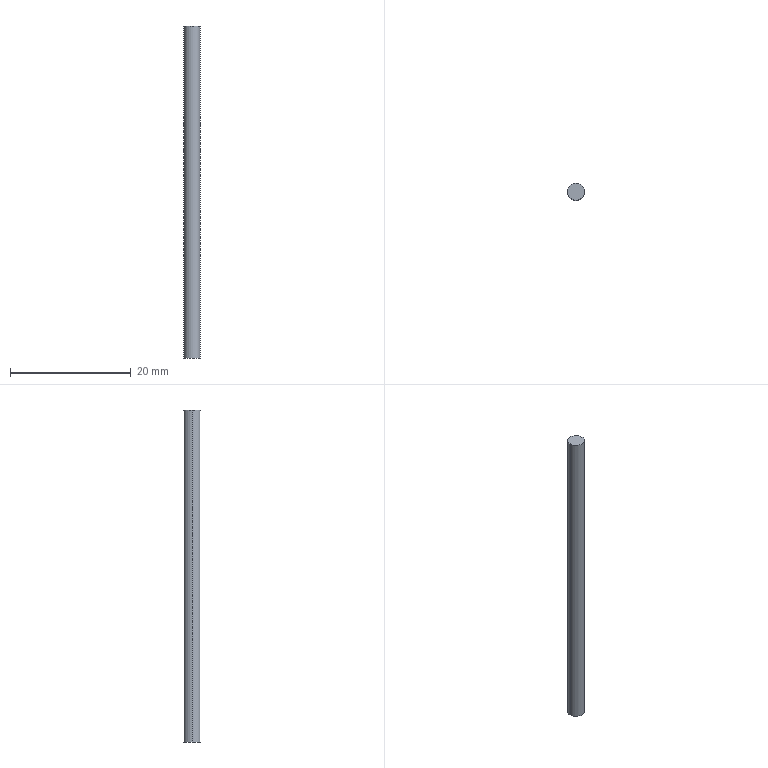Part | SolidWorks | features Extrusion 1 | 1 solid | 4 faces | box 2.8 x 2.8 x 55 mm | volume 338.664 mm3 | cylinder 2 | plane 2 | commonest cylinder face diameters 2.8 x2
STEP:
#1=CARTESIAN_POINT('',(-149.719,-87.732,27.5));
#2=VERTEX_POINT('',#1);
#3=CARTESIAN_POINT('',(-152.519,-87.732,27.5));
#4=VERTEX_POINT('',#3);
#5=CARTESIAN_POINT('',(-151.119,-87.732,27.5));
#6=DIRECTION('',(0.,0.,1.));
#7=DIRECTION('',(1.,0.,0.));
#8=AXIS2_PLACEMENT_3D('',#5,#6,#7);
#9=CIRCLE('',#8,1.4);
#10=EDGE_CURVE('',#2,#4,#9,.T.);
#11=ORIENTED_EDGE('',*,*,#10,.F.);
#12=CARTESIAN_POINT('',(-149.719,-87.732,-27.5));
#13=VERTEX_POINT('',#12);
#14=CARTESIAN_POINT('',(-149.719,-87.732,27.5));
#15=DIRECTION('',(0.,0.,-1.));
#16=VECTOR('',#15,1000.);
#17=LINE('',#14,#16);
#18=EDGE_CURVE('',#2,#13,#17,.T.);
#19=ORIENTED_EDGE('',*,*,#18,.T.);
#20=CARTESIAN_POINT('',(-152.519,-87.732,-27.5));
#21=VERTEX_POINT('',#20);
#22=CARTESIAN_POINT('',(-151.119,-87.732,-27.5));
#23=DIRECTION('',(0.,0.,1.));
#24=DIRECTION('',(1.,0.,0.));
#25=AXIS2_PLACEMENT_3D('',#22,#23,#24);
#26=CIRCLE('',#25,1.4);
#27=EDGE_CURVE('',#13,#21,#26,.T.);
#28=ORIENTED_EDGE('',*,*,#27,.T.);
#29=CARTESIAN_POINT('',(-152.519,-87.732,27.5));
#30=DIRECTION('',(0.,0.,-1.));
#31=VECTOR('',#30,1000.);
#32=LINE('',#29,#31);
#33=EDGE_CURVE('',#4,#21,#32,.T.);
#34=ORIENTED_EDGE('',*,*,#33,.F.);
#35=EDGE_LOOP('',(#11,#19,#28,#34));
#36=FACE_OUTER_BOUND('',#35,.T.);
#37=CARTESIAN_POINT('',(-151.119,-87.732,27.5));
#38=DIRECTION('',(0.,0.,-1.));
#39=DIRECTION('',(-1.,0.,0.));
#40=AXIS2_PLACEMENT_3D('',#37,#38,#39);
#41=CYLINDRICAL_SURFACE('',#40,1.4);
#42=ADVANCED_FACE('',(#36),#41,.T.);
#43=ORIENTED_EDGE('',*,*,#18,.F.);
#44=CARTESIAN_POINT('',(-151.119,-87.732,27.5));
#45=DIRECTION('',(0.,0.,1.));
#46=DIRECTION('',(1.,0.,0.));
#47=AXIS2_PLACEMENT_3D('',#44,#45,#46);
#48=CIRCLE('',#47,1.4);
#49=EDGE_CURVE('',#4,#2,#48,.T.);
#50=ORIENTED_EDGE('',*,*,#49,.F.);
#51=ORIENTED_EDGE('',*,*,#33,.T.);
#52=CARTESIAN_POINT('',(-151.119,-87.732,-27.5));
#53=DIRECTION('',(0.,0.,1.));
#54=DIRECTION('',(1.,0.,0.));
#55=AXIS2_PLACEMENT_3D('',#52,#53,#54);
#56=CIRCLE('',#55,1.4);
#57=EDGE_CURVE('',#21,#13,#56,.T.);
#58=ORIENTED_EDGE('',*,*,#57,.T.);
#59=EDGE_LOOP('',(#43,#50,#51,#58));
#60=FACE_OUTER_BOUND('',#59,.T.);
#61=CARTESIAN_POINT('',(-151.119,-87.732,27.5));
#62=DIRECTION('',(0.,0.,-1.));
#63=DIRECTION('',(-1.,0.,0.));
#64=AXIS2_PLACEMENT_3D('',#61,#62,#63);
#65=CYLINDRICAL_SURFACE('',#64,1.4);
#66=ADVANCED_FACE('',(#60),#65,.T.);
#67=ORIENTED_EDGE('',*,*,#49,.T.);
#68=ORIENTED_EDGE('',*,*,#10,.T.);
#69=EDGE_LOOP('',(#67,#68));
#70=FACE_OUTER_BOUND('',#69,.T.);
#71=CARTESIAN_POINT('',(-151.119,-87.732,27.5));
#72=DIRECTION('',(0.,0.,1.));
#73=DIRECTION('',(1.,0.,0.));
#74=AXIS2_PLACEMENT_3D('',#71,#72,#73);
#75=PLANE('',#74);
#76=ADVANCED_FACE('',(#70),#75,.T.);
#77=ORIENTED_EDGE('',*,*,#57,.F.);
#78=ORIENTED_EDGE('',*,*,#27,.F.);
#79=EDGE_LOOP('',(#77,#78));
#80=FACE_OUTER_BOUND('',#79,.T.);
#81=CARTESIAN_POINT('',(-151.119,-87.732,-27.5));
#82=DIRECTION('',(0.,0.,1.));
#83=DIRECTION('',(1.,0.,0.));
#84=AXIS2_PLACEMENT_3D('',#81,#82,#83);
#85=PLANE('',#84);
#86=ADVANCED_FACE('',(#80),#85,.F.);
#87=CLOSED_SHELL('',(#42,#66,#76,#86));
#88=MANIFOLD_SOLID_BREP('',#87);
#89=CARTESIAN_POINT('',(0.,0.,0.));
#90=DIRECTION('',(0.,0.,1.));
#91=DIRECTION('',(1.,0.,0.));
#92=AXIS2_PLACEMENT_3D('',#89,#90,#91);
#93=(LENGTH_UNIT()NAMED_UNIT(*)SI_UNIT(.MILLI.,.METRE.));
#94=UNCERTAINTY_MEASURE_WITH_UNIT(LENGTH_MEASURE(0.00001),#93,'','');
#95=(NAMED_UNIT(*)PLANE_ANGLE_UNIT()SI_UNIT($,.RADIAN.));
#96=(NAMED_UNIT(*)SI_UNIT($,.STERADIAN.)SOLID_ANGLE_UNIT());
#97=(GEOMETRIC_REPRESENTATION_CONTEXT(3)GLOBAL_UNCERTAINTY_ASSIGNED_CONTEXT((#94))GLOBAL_UNIT_ASSIGNED_CONTEXT((#93,#95,#96))REPRESENTATION_CONTEXT('',''));
#98=ADVANCED_BREP_SHAPE_REPRESENTATION('',(#88,#92),#97);